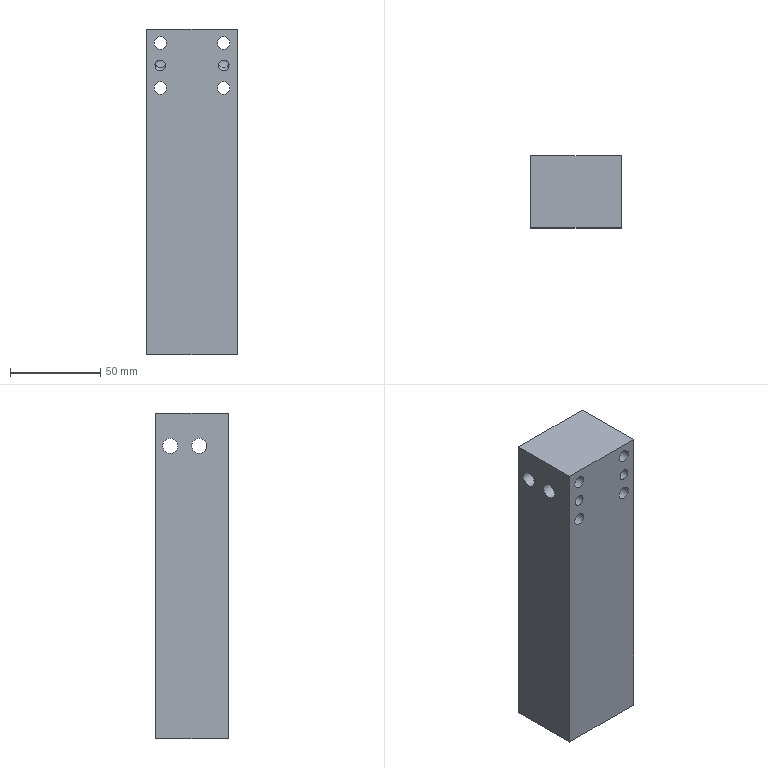Part | NX | features BREP 1 | 1 solid | 24 faces | box 50 x 40 x 180 mm | volume 345283 mm3 | cylinder 12 | plane 6 | cone 6 | commonest cylinder face diameters 6 x4 7 x4 6.8 x2 8.5 x2
STEP:
#1=CARTESIAN_POINT('',(25.,12.,67.75));
#2=VERTEX_POINT('',#1);
#3=CARTESIAN_POINT('',(25.,12.,72.));
#4=DIRECTION('',(1.,0.,0.));
#5=DIRECTION('',(0.,0.,-1.));
#6=AXIS2_PLACEMENT_3D('',#3,#4,#5);
#7=CIRCLE('',#6,4.25);
#8=EDGE_CURVE('',#2,#2,#7,.T.);
#9=ORIENTED_EDGE('',*,*,#8,.F.);
#10=EDGE_LOOP('',(#9));
#11=FACE_BOUND('',#10,.T.);
#12=CARTESIAN_POINT('',(25.,-4.,67.75));
#13=VERTEX_POINT('',#12);
#14=CARTESIAN_POINT('',(25.,-4.,72.));
#15=DIRECTION('',(1.,0.,0.));
#16=DIRECTION('',(0.,0.,-1.));
#17=AXIS2_PLACEMENT_3D('',#14,#15,#16);
#18=CIRCLE('',#17,4.25);
#19=EDGE_CURVE('',#13,#13,#18,.T.);
#20=ORIENTED_EDGE('',*,*,#19,.F.);
#21=EDGE_LOOP('',(#20));
#22=FACE_BOUND('',#21,.T.);
#23=CARTESIAN_POINT('',(25.,-20.,90.));
#24=VERTEX_POINT('',#23);
#25=CARTESIAN_POINT('',(25.,-20.,-90.));
#26=VERTEX_POINT('',#25);
#27=CARTESIAN_POINT('',(25.,-20.,90.));
#28=DIRECTION('',(0.,0.,-1.));
#29=VECTOR('',#28,1000.);
#30=LINE('',#27,#29);
#31=EDGE_CURVE('',#24,#26,#30,.T.);
#32=ORIENTED_EDGE('',*,*,#31,.T.);
#33=CARTESIAN_POINT('',(25.,20.,-90.));
#34=VERTEX_POINT('',#33);
#35=CARTESIAN_POINT('',(25.,20.,-90.));
#36=DIRECTION('',(0.,-1.,0.));
#37=VECTOR('',#36,1000.);
#38=LINE('',#35,#37);
#39=EDGE_CURVE('',#34,#26,#38,.T.);
#40=ORIENTED_EDGE('',*,*,#39,.F.);
#41=CARTESIAN_POINT('',(25.,20.,90.));
#42=VERTEX_POINT('',#41);
#43=CARTESIAN_POINT('',(25.,20.,90.));
#44=DIRECTION('',(0.,0.,-1.));
#45=VECTOR('',#44,1000.);
#46=LINE('',#43,#45);
#47=EDGE_CURVE('',#42,#34,#46,.T.);
#48=ORIENTED_EDGE('',*,*,#47,.F.);
#49=CARTESIAN_POINT('',(25.,20.,90.));
#50=DIRECTION('',(0.,-1.,0.));
#51=VECTOR('',#50,1000.);
#52=LINE('',#49,#51);
#53=EDGE_CURVE('',#42,#24,#52,.T.);
#54=ORIENTED_EDGE('',*,*,#53,.T.);
#55=EDGE_LOOP('',(#32,#40,#48,#54));
#56=FACE_BOUND('',#55,.T.);
#57=CARTESIAN_POINT('',(25.,20.,90.));
#58=DIRECTION('',(-1.,0.,0.));
#59=DIRECTION('',(0.,0.,-1.));
#60=AXIS2_PLACEMENT_3D('',#57,#58,#59);
#61=PLANE('',#60);
#62=ADVANCED_FACE('',(#11,#22,#56),#61,.F.);
#63=CARTESIAN_POINT('',(9.5,10.,-90.));
#64=VERTEX_POINT('',#63);
#65=CARTESIAN_POINT('',(12.5,10.,-90.));
#66=DIRECTION('',(0.,0.,-1.));
#67=DIRECTION('',(-1.,0.,0.));
#68=AXIS2_PLACEMENT_3D('',#65,#66,#67);
#69=CIRCLE('',#68,3.);
#70=EDGE_CURVE('',#64,#64,#69,.T.);
#71=ORIENTED_EDGE('',*,*,#70,.F.);
#72=EDGE_LOOP('',(#71));
#73=FACE_BOUND('',#72,.T.);
#74=CARTESIAN_POINT('',(-15.5,-10.,-90.));
#75=VERTEX_POINT('',#74);
#76=CARTESIAN_POINT('',(-12.5,-10.,-90.));
#77=DIRECTION('',(0.,0.,-1.));
#78=DIRECTION('',(-1.,0.,0.));
#79=AXIS2_PLACEMENT_3D('',#76,#77,#78);
#80=CIRCLE('',#79,3.);
#81=EDGE_CURVE('',#75,#75,#80,.T.);
#82=ORIENTED_EDGE('',*,*,#81,.F.);
#83=EDGE_LOOP('',(#82));
#84=FACE_BOUND('',#83,.T.);
#85=CARTESIAN_POINT('',(-15.9,10.,-90.));
#86=VERTEX_POINT('',#85);
#87=CARTESIAN_POINT('',(-12.5,10.,-90.));
#88=DIRECTION('',(0.,0.,-1.));
#89=DIRECTION('',(-1.,0.,0.));
#90=AXIS2_PLACEMENT_3D('',#87,#88,#89);
#91=CIRCLE('',#90,3.4);
#92=EDGE_CURVE('',#86,#86,#91,.T.);
#93=ORIENTED_EDGE('',*,*,#92,.F.);
#94=EDGE_LOOP('',(#93));
#95=FACE_BOUND('',#94,.T.);
#96=CARTESIAN_POINT('',(9.1,-10.,-90.));
#97=VERTEX_POINT('',#96);
#98=CARTESIAN_POINT('',(12.5,-10.,-90.));
#99=DIRECTION('',(0.,0.,-1.));
#100=DIRECTION('',(-1.,0.,0.));
#101=AXIS2_PLACEMENT_3D('',#98,#99,#100);
#102=CIRCLE('',#101,3.4);
#103=EDGE_CURVE('',#97,#97,#102,.T.);
#104=ORIENTED_EDGE('',*,*,#103,.F.);
#105=EDGE_LOOP('',(#104));
#106=FACE_BOUND('',#105,.T.);
#107=CARTESIAN_POINT('',(-25.,-20.,-90.));
#108=VERTEX_POINT('',#107);
#109=CARTESIAN_POINT('',(-25.,-20.,-90.));
#110=DIRECTION('',(-1.,0.,0.));
#111=VECTOR('',#110,1000.);
#112=LINE('',#109,#111);
#113=EDGE_CURVE('',#26,#108,#112,.T.);
#114=ORIENTED_EDGE('',*,*,#113,.T.);
#115=CARTESIAN_POINT('',(-25.,20.,-90.));
#116=VERTEX_POINT('',#115);
#117=CARTESIAN_POINT('',(-25.,20.,-90.));
#118=DIRECTION('',(0.,-1.,0.));
#119=VECTOR('',#118,1000.);
#120=LINE('',#117,#119);
#121=EDGE_CURVE('',#116,#108,#120,.T.);
#122=ORIENTED_EDGE('',*,*,#121,.F.);
#123=CARTESIAN_POINT('',(-25.,20.,-90.));
#124=DIRECTION('',(-1.,0.,0.));
#125=VECTOR('',#124,1000.);
#126=LINE('',#123,#125);
#127=EDGE_CURVE('',#34,#116,#126,.T.);
#128=ORIENTED_EDGE('',*,*,#127,.F.);
#129=ORIENTED_EDGE('',*,*,#39,.T.);
#130=EDGE_LOOP('',(#114,#122,#128,#129));
#131=FACE_BOUND('',#130,.T.);
#132=CARTESIAN_POINT('',(-25.,20.,-90.));
#133=DIRECTION('',(0.,0.,1.));
#134=DIRECTION('',(-1.,0.,0.));
#135=AXIS2_PLACEMENT_3D('',#132,#133,#134);
#136=PLANE('',#135);
#137=ADVANCED_FACE('',(#73,#84,#95,#106,#131),#136,.F.);
#138=CARTESIAN_POINT('',(-25.,12.,67.75));
#139=VERTEX_POINT('',#138);
#140=CARTESIAN_POINT('',(-25.,12.,72.));
#141=DIRECTION('',(1.,0.,0.));
#142=DIRECTION('',(0.,0.,-1.));
#143=AXIS2_PLACEMENT_3D('',#140,#141,#142);
#144=CIRCLE('',#143,4.25);
#145=EDGE_CURVE('',#139,#139,#144,.T.);
#146=ORIENTED_EDGE('',*,*,#145,.T.);
#147=EDGE_LOOP('',(#146));
#148=FACE_BOUND('',#147,.T.);
#149=CARTESIAN_POINT('',(-25.,-4.,67.75));
#150=VERTEX_POINT('',#149);
#151=CARTESIAN_POINT('',(-25.,-4.,72.));
#152=DIRECTION('',(1.,0.,0.));
#153=DIRECTION('',(0.,0.,-1.));
#154=AXIS2_PLACEMENT_3D('',#151,#152,#153);
#155=CIRCLE('',#154,4.25);
#156=EDGE_CURVE('',#150,#150,#155,.T.);
#157=ORIENTED_EDGE('',*,*,#156,.T.);
#158=EDGE_LOOP('',(#157));
#159=FACE_BOUND('',#158,.T.);
#160=CARTESIAN_POINT('',(-25.,-20.,90.));
#161=VERTEX_POINT('',#160);
#162=CARTESIAN_POINT('',(-25.,-20.,90.));
#163=DIRECTION('',(0.,0.,1.));
#164=VECTOR('',#163,1000.);
#165=LINE('',#162,#164);
#166=EDGE_CURVE('',#108,#161,#165,.T.);
#167=ORIENTED_EDGE('',*,*,#166,.T.);
#168=CARTESIAN_POINT('',(-25.,20.,90.));
#169=VERTEX_POINT('',#168);
#170=CARTESIAN_POINT('',(-25.,20.,90.));
#171=DIRECTION('',(0.,-1.,0.));
#172=VECTOR('',#171,1000.);
#173=LINE('',#170,#172);
#174=EDGE_CURVE('',#169,#161,#173,.T.);
#175=ORIENTED_EDGE('',*,*,#174,.F.);
#176=CARTESIAN_POINT('',(-25.,20.,90.));
#177=DIRECTION('',(0.,0.,1.));
#178=VECTOR('',#177,1000.);
#179=LINE('',#176,#178);
#180=EDGE_CURVE('',#116,#169,#179,.T.);
#181=ORIENTED_EDGE('',*,*,#180,.F.);
#182=ORIENTED_EDGE('',*,*,#121,.T.);
#183=EDGE_LOOP('',(#167,#175,#181,#182));
#184=FACE_BOUND('',#183,.T.);
#185=CARTESIAN_POINT('',(-25.,20.,90.));
#186=DIRECTION('',(1.,0.,0.));
#187=DIRECTION('',(0.,0.,1.));
#188=AXIS2_PLACEMENT_3D('',#185,#186,#187);
#189=PLANE('',#188);
#190=ADVANCED_FACE('',(#148,#159,#184),#189,.F.);
#191=CARTESIAN_POINT('',(-25.,-20.,90.));
#192=DIRECTION('',(1.,0.,0.));
#193=VECTOR('',#192,1000.);
#194=LINE('',#191,#193);
#195=EDGE_CURVE('',#161,#24,#194,.T.);
#196=ORIENTED_EDGE('',*,*,#195,.T.);
#197=ORIENTED_EDGE('',*,*,#53,.F.);
#198=CARTESIAN_POINT('',(-25.,20.,90.));
#199=DIRECTION('',(1.,0.,0.));
#200=VECTOR('',#199,1000.);
#201=LINE('',#198,#200);
#202=EDGE_CURVE('',#169,#42,#201,.T.);
#203=ORIENTED_EDGE('',*,*,#202,.F.);
#204=ORIENTED_EDGE('',*,*,#174,.T.);
#205=EDGE_LOOP('',(#196,#197,#203,#204));
#206=FACE_BOUND('',#205,.T.);
#207=CARTESIAN_POINT('',(-25.,20.,90.));
#208=DIRECTION('',(0.,0.,-1.));
#209=DIRECTION('',(1.,0.,0.));
#210=AXIS2_PLACEMENT_3D('',#207,#208,#209);
#211=PLANE('',#210);
#212=ADVANCED_FACE('',(#206),#211,.F.);
#213=CARTESIAN_POINT('',(17.5,20.,86.));
#214=VERTEX_POINT('',#213);
#215=CARTESIAN_POINT('',(17.5,20.,82.5));
#216=DIRECTION('',(0.,1.,0.));
#217=DIRECTION('',(0.,0.,1.));
#218=AXIS2_PLACEMENT_3D('',#215,#216,#217);
#219=CIRCLE('',#218,3.5);
#220=EDGE_CURVE('',#214,#214,#219,.T.);
#221=ORIENTED_EDGE('',*,*,#220,.F.);
#222=EDGE_LOOP('',(#221));
#223=FACE_BOUND('',#222,.T.);
#224=CARTESIAN_POINT('',(17.5,20.,61.));
#225=VERTEX_POINT('',#224);
#226=CARTESIAN_POINT('',(17.5,20.,57.5));
#227=DIRECTION('',(0.,1.,0.));
#228=DIRECTION('',(0.,0.,1.));
#229=AXIS2_PLACEMENT_3D('',#226,#227,#228);
#230=CIRCLE('',#229,3.5);
#231=EDGE_CURVE('',#225,#225,#230,.T.);
#232=ORIENTED_EDGE('',*,*,#231,.F.);
#233=EDGE_LOOP('',(#232));
#234=FACE_BOUND('',#233,.T.);
#235=CARTESIAN_POINT('',(-17.5,20.,61.));
#236=VERTEX_POINT('',#235);
#237=CARTESIAN_POINT('',(-17.5,20.,57.5));
#238=DIRECTION('',(0.,1.,0.));
#239=DIRECTION('',(0.,0.,1.));
#240=AXIS2_PLACEMENT_3D('',#237,#238,#239);
#241=CIRCLE('',#240,3.5);
#242=EDGE_CURVE('',#236,#236,#241,.T.);
#243=ORIENTED_EDGE('',*,*,#242,.F.);
#244=EDGE_LOOP('',(#243));
#245=FACE_BOUND('',#244,.T.);
#246=CARTESIAN_POINT('',(-17.5,20.,86.));
#247=VERTEX_POINT('',#246);
#248=CARTESIAN_POINT('',(-17.5,20.,82.5));
#249=DIRECTION('',(0.,1.,0.));
#250=DIRECTION('',(0.,0.,1.));
#251=AXIS2_PLACEMENT_3D('',#248,#249,#250);
#252=CIRCLE('',#251,3.5);
#253=EDGE_CURVE('',#247,#247,#252,.T.);
#254=ORIENTED_EDGE('',*,*,#253,.F.);
#255=EDGE_LOOP('',(#254));
#256=FACE_BOUND('',#255,.T.);
#257=ORIENTED_EDGE('',*,*,#47,.T.);
#258=ORIENTED_EDGE('',*,*,#127,.T.);
#259=ORIENTED_EDGE('',*,*,#180,.T.);
#260=ORIENTED_EDGE('',*,*,#202,.T.);
#261=EDGE_LOOP('',(#257,#258,#259,#260));
#262=FACE_BOUND('',#261,.T.);
#263=CARTESIAN_POINT('',(0.,20.,0.));
#264=DIRECTION('',(0.,-1.,0.));
#265=DIRECTION('',(0.,0.,1.));
#266=AXIS2_PLACEMENT_3D('',#263,#264,#265);
#267=PLANE('',#266);
#268=ADVANCED_FACE('',(#223,#234,#245,#256,#262),#267,.F.);
#269=CARTESIAN_POINT('',(-17.5,-20.,67.));
#270=VERTEX_POINT('',#269);
#271=CARTESIAN_POINT('',(-17.5,-20.,70.));
#272=DIRECTION('',(0.,-1.,0.));
#273=DIRECTION('',(0.,0.,-1.));
#274=AXIS2_PLACEMENT_3D('',#271,#272,#273);
#275=CIRCLE('',#274,3.);
#276=EDGE_CURVE('',#270,#270,#275,.T.);
#277=ORIENTED_EDGE('',*,*,#276,.F.);
#278=EDGE_LOOP('',(#277));
#279=FACE_BOUND('',#278,.T.);
#280=CARTESIAN_POINT('',(17.5,-20.,67.));
#281=VERTEX_POINT('',#280);
#282=CARTESIAN_POINT('',(17.5,-20.,70.));
#283=DIRECTION('',(0.,-1.,0.));
#284=DIRECTION('',(0.,0.,-1.));
#285=AXIS2_PLACEMENT_3D('',#282,#283,#284);
#286=CIRCLE('',#285,3.);
#287=EDGE_CURVE('',#281,#281,#286,.T.);
#288=ORIENTED_EDGE('',*,*,#287,.F.);
#289=EDGE_LOOP('',(#288));
#290=FACE_BOUND('',#289,.T.);
#291=CARTESIAN_POINT('',(17.5,-20.,86.));
#292=VERTEX_POINT('',#291);
#293=CARTESIAN_POINT('',(17.5,-20.,82.5));
#294=DIRECTION('',(0.,1.,0.));
#295=DIRECTION('',(0.,0.,1.));
#296=AXIS2_PLACEMENT_3D('',#293,#294,#295);
#297=CIRCLE('',#296,3.5);
#298=EDGE_CURVE('',#292,#292,#297,.T.);
#299=ORIENTED_EDGE('',*,*,#298,.T.);
#300=EDGE_LOOP('',(#299));
#301=FACE_BOUND('',#300,.T.);
#302=CARTESIAN_POINT('',(17.5,-20.,61.));
#303=VERTEX_POINT('',#302);
#304=CARTESIAN_POINT('',(17.5,-20.,57.5));
#305=DIRECTION('',(0.,1.,0.));
#306=DIRECTION('',(0.,0.,1.));
#307=AXIS2_PLACEMENT_3D('',#304,#305,#306);
#308=CIRCLE('',#307,3.5);
#309=EDGE_CURVE('',#303,#303,#308,.T.);
#310=ORIENTED_EDGE('',*,*,#309,.T.);
#311=EDGE_LOOP('',(#310));
#312=FACE_BOUND('',#311,.T.);
#313=CARTESIAN_POINT('',(-17.5,-20.,61.));
#314=VERTEX_POINT('',#313);
#315=CARTESIAN_POINT('',(-17.5,-20.,57.5));
#316=DIRECTION('',(0.,1.,0.));
#317=DIRECTION('',(0.,0.,1.));
#318=AXIS2_PLACEMENT_3D('',#315,#316,#317);
#319=CIRCLE('',#318,3.5);
#320=EDGE_CURVE('',#314,#314,#319,.T.);
#321=ORIENTED_EDGE('',*,*,#320,.T.);
#322=EDGE_LOOP('',(#321));
#323=FACE_BOUND('',#322,.T.);
#324=CARTESIAN_POINT('',(-17.5,-20.,86.));
#325=VERTEX_POINT('',#324);
#326=CARTESIAN_POINT('',(-17.5,-20.,82.5));
#327=DIRECTION('',(0.,1.,0.));
#328=DIRECTION('',(0.,0.,1.));
#329=AXIS2_PLACEMENT_3D('',#326,#327,#328);
#330=CIRCLE('',#329,3.5);
#331=EDGE_CURVE('',#325,#325,#330,.T.);
#332=ORIENTED_EDGE('',*,*,#331,.T.);
#333=EDGE_LOOP('',(#332));
#334=FACE_BOUND('',#333,.T.);
#335=ORIENTED_EDGE('',*,*,#31,.F.);
#336=ORIENTED_EDGE('',*,*,#195,.F.);
#337=ORIENTED_EDGE('',*,*,#166,.F.);
#338=ORIENTED_EDGE('',*,*,#113,.F.);
#339=EDGE_LOOP('',(#335,#336,#337,#338));
#340=FACE_BOUND('',#339,.T.);
#341=CARTESIAN_POINT('',(0.,-20.,0.));
#342=DIRECTION('',(0.,-1.,0.));
#343=DIRECTION('',(0.,0.,1.));
#344=AXIS2_PLACEMENT_3D('',#341,#342,#343);
#345=PLANE('',#344);
#346=ADVANCED_FACE('',(#279,#290,#301,#312,#323,#334,#340),#345,.T.);
#347=ORIENTED_EDGE('',*,*,#331,.F.);
#348=EDGE_LOOP('',(#347));
#349=FACE_BOUND('',#348,.T.);
#350=ORIENTED_EDGE('',*,*,#253,.T.);
#351=EDGE_LOOP('',(#350));
#352=FACE_BOUND('',#351,.T.);
#353=CARTESIAN_POINT('',(-17.5,20.,82.5));
#354=DIRECTION('',(0.,1.,0.));
#355=DIRECTION('',(0.,0.,-1.));
#356=AXIS2_PLACEMENT_3D('',#353,#354,#355);
#357=CYLINDRICAL_SURFACE('',#356,3.5);
#358=ADVANCED_FACE('',(#349,#352),#357,.F.);
#359=ORIENTED_EDGE('',*,*,#320,.F.);
#360=EDGE_LOOP('',(#359));
#361=FACE_BOUND('',#360,.T.);
#362=ORIENTED_EDGE('',*,*,#242,.T.);
#363=EDGE_LOOP('',(#362));
#364=FACE_BOUND('',#363,.T.);
#365=CARTESIAN_POINT('',(-17.5,20.,57.5));
#366=DIRECTION('',(0.,1.,0.));
#367=DIRECTION('',(0.,0.,-1.));
#368=AXIS2_PLACEMENT_3D('',#365,#366,#367);
#369=CYLINDRICAL_SURFACE('',#368,3.5);
#370=ADVANCED_FACE('',(#361,#364),#369,.F.);
#371=ORIENTED_EDGE('',*,*,#309,.F.);
#372=EDGE_LOOP('',(#371));
#373=FACE_BOUND('',#372,.T.);
#374=ORIENTED_EDGE('',*,*,#231,.T.);
#375=EDGE_LOOP('',(#374));
#376=FACE_BOUND('',#375,.T.);
#377=CARTESIAN_POINT('',(17.5,20.,57.5));
#378=DIRECTION('',(0.,1.,0.));
#379=DIRECTION('',(0.,0.,-1.));
#380=AXIS2_PLACEMENT_3D('',#377,#378,#379);
#381=CYLINDRICAL_SURFACE('',#380,3.5);
#382=ADVANCED_FACE('',(#373,#376),#381,.F.);
#383=ORIENTED_EDGE('',*,*,#298,.F.);
#384=EDGE_LOOP('',(#383));
#385=FACE_BOUND('',#384,.T.);
#386=ORIENTED_EDGE('',*,*,#220,.T.);
#387=EDGE_LOOP('',(#386));
#388=FACE_BOUND('',#387,.T.);
#389=CARTESIAN_POINT('',(17.5,20.,82.5));
#390=DIRECTION('',(0.,1.,0.));
#391=DIRECTION('',(0.,0.,-1.));
#392=AXIS2_PLACEMENT_3D('',#389,#390,#391);
#393=CYLINDRICAL_SURFACE('',#392,3.5);
#394=ADVANCED_FACE('',(#385,#388),#393,.F.);
#395=CARTESIAN_POINT('',(12.5,-10.,-68.207));
#396=VERTEX_POINT('',#395);
#397=VERTEX_LOOP('',#396);
#398=FACE_BOUND('',#397,.T.);
#399=CARTESIAN_POINT('',(9.1,-10.,-70.25));
#400=VERTEX_POINT('',#399);
#401=CARTESIAN_POINT('',(12.5,-10.,-70.25));
#402=DIRECTION('',(0.,0.,-1.));
#403=DIRECTION('',(-1.,0.,0.));
#404=AXIS2_PLACEMENT_3D('',#401,#402,#403);
#405=CIRCLE('',#404,3.4);
#406=EDGE_CURVE('',#400,#400,#405,.T.);
#407=ORIENTED_EDGE('',*,*,#406,.T.);
#408=EDGE_LOOP('',(#407));
#409=FACE_BOUND('',#408,.T.);
#410=CARTESIAN_POINT('',(12.5,-10.,-70.25));
#411=DIRECTION('',(0.,0.,-1.));
#412=DIRECTION('',(1.,0.,0.));
#413=AXIS2_PLACEMENT_3D('',#410,#411,#412);
#414=CONICAL_SURFACE('',#413,3.4,1.03);
#415=ADVANCED_FACE('',(#398,#409),#414,.F.);
#416=ORIENTED_EDGE('',*,*,#406,.F.);
#417=EDGE_LOOP('',(#416));
#418=FACE_BOUND('',#417,.T.);
#419=ORIENTED_EDGE('',*,*,#103,.T.);
#420=EDGE_LOOP('',(#419));
#421=FACE_BOUND('',#420,.T.);
#422=CARTESIAN_POINT('',(12.5,-10.,-90.));
#423=DIRECTION('',(0.,0.,-1.));
#424=DIRECTION('',(1.,0.,0.));
#425=AXIS2_PLACEMENT_3D('',#422,#423,#424);
#426=CYLINDRICAL_SURFACE('',#425,3.4);
#427=ADVANCED_FACE('',(#418,#421),#426,.F.);
#428=CARTESIAN_POINT('',(-12.5,10.,-68.207));
#429=VERTEX_POINT('',#428);
#430=VERTEX_LOOP('',#429);
#431=FACE_BOUND('',#430,.T.);
#432=CARTESIAN_POINT('',(-15.9,10.,-70.25));
#433=VERTEX_POINT('',#432);
#434=CARTESIAN_POINT('',(-12.5,10.,-70.25));
#435=DIRECTION('',(0.,0.,-1.));
#436=DIRECTION('',(-1.,0.,0.));
#437=AXIS2_PLACEMENT_3D('',#434,#435,#436);
#438=CIRCLE('',#437,3.4);
#439=EDGE_CURVE('',#433,#433,#438,.T.);
#440=ORIENTED_EDGE('',*,*,#439,.T.);
#441=EDGE_LOOP('',(#440));
#442=FACE_BOUND('',#441,.T.);
#443=CARTESIAN_POINT('',(-12.5,10.,-70.25));
#444=DIRECTION('',(0.,0.,-1.));
#445=DIRECTION('',(1.,0.,0.));
#446=AXIS2_PLACEMENT_3D('',#443,#444,#445);
#447=CONICAL_SURFACE('',#446,3.4,1.03);
#448=ADVANCED_FACE('',(#431,#442),#447,.F.);
#449=ORIENTED_EDGE('',*,*,#439,.F.);
#450=EDGE_LOOP('',(#449));
#451=FACE_BOUND('',#450,.T.);
#452=ORIENTED_EDGE('',*,*,#92,.T.);
#453=EDGE_LOOP('',(#452));
#454=FACE_BOUND('',#453,.T.);
#455=CARTESIAN_POINT('',(-12.5,10.,-90.));
#456=DIRECTION('',(0.,0.,-1.));
#457=DIRECTION('',(1.,0.,0.));
#458=AXIS2_PLACEMENT_3D('',#455,#456,#457);
#459=CYLINDRICAL_SURFACE('',#458,3.4);
#460=ADVANCED_FACE('',(#451,#454),#459,.F.);
#461=CARTESIAN_POINT('',(14.553,-8.,70.564));
#462=VERTEX_POINT('',#461);
#463=CARTESIAN_POINT('',(20.447,-8.,70.564));
#464=VERTEX_POINT('',#463);
#465=CARTESIAN_POINT('',(17.5,-8.,70.));
#466=DIRECTION('',(0.,-1.,0.));
#467=DIRECTION('',(0.,0.,-1.));
#468=AXIS2_PLACEMENT_3D('',#465,#466,#467);
#469=CIRCLE('',#468,3.);
#470=EDGE_CURVE('',#462,#464,#469,.T.);
#471=ORIENTED_EDGE('',*,*,#470,.T.);
#472=CARTESIAN_POINT('',(20.447,-8.,70.564));
#473=CARTESIAN_POINT('',(20.214,-7.8,70.007));
#474=CARTESIAN_POINT('',(19.317,-7.293,69.243));
#475=CARTESIAN_POINT('',(17.511,-6.669,68.686));
#476=CARTESIAN_POINT('',(15.688,-7.288,69.237));
#477=CARTESIAN_POINT('',(14.786,-7.8,70.006));
#478=CARTESIAN_POINT('',(14.553,-8.,70.564));
#479=B_SPLINE_CURVE_WITH_KNOTS('',3,(#472,#473,#474,#475,#476,#477,#478),.UNSPECIFIED.,.F.,.F.,(4,1,1,1,4),(0.,0.001872,0.003744,0.005615,0.007487),.UNSPECIFIED.);
#480=EDGE_CURVE('',#464,#462,#479,.T.);
#481=ORIENTED_EDGE('',*,*,#480,.T.);
#482=EDGE_LOOP('',(#471,#481));
#483=FACE_BOUND('',#482,.T.);
#484=CARTESIAN_POINT('',(17.5,-8.,70.));
#485=DIRECTION('',(0.,-1.,0.));
#486=DIRECTION('',(0.,0.,1.));
#487=AXIS2_PLACEMENT_3D('',#484,#485,#486);
#488=CONICAL_SURFACE('',#487,3.,1.03);
#489=ADVANCED_FACE('',(#483),#488,.F.);
#490=ORIENTED_EDGE('',*,*,#470,.F.);
#491=CARTESIAN_POINT('',(14.553,-8.,70.564));
#492=CARTESIAN_POINT('',(14.678,-8.234,71.215));
#493=CARTESIAN_POINT('',(15.418,-8.296,72.503));
#494=CARTESIAN_POINT('',(17.501,-8.048,73.249));
#495=CARTESIAN_POINT('',(19.582,-8.296,72.503));
#496=CARTESIAN_POINT('',(20.322,-8.234,71.215));
#497=CARTESIAN_POINT('',(20.447,-8.,70.564));
#498=B_SPLINE_CURVE_WITH_KNOTS('',3,(#491,#492,#493,#494,#495,#496,#497),.UNSPECIFIED.,.F.,.F.,(4,1,1,1,4),(0.,0.002078,0.004155,0.006233,0.008311),.UNSPECIFIED.);
#499=EDGE_CURVE('',#462,#464,#498,.T.);
#500=ORIENTED_EDGE('',*,*,#499,.T.);
#501=EDGE_LOOP('',(#490,#500));
#502=FACE_BOUND('',#501,.T.);
#503=ORIENTED_EDGE('',*,*,#287,.T.);
#504=EDGE_LOOP('',(#503));
#505=FACE_BOUND('',#504,.T.);
#506=CARTESIAN_POINT('',(17.5,-20.,70.));
#507=DIRECTION('',(0.,-1.,0.));
#508=DIRECTION('',(0.,0.,1.));
#509=AXIS2_PLACEMENT_3D('',#506,#507,#508);
#510=CYLINDRICAL_SURFACE('',#509,3.);
#511=ADVANCED_FACE('',(#502,#505),#510,.F.);
#512=CARTESIAN_POINT('',(-20.447,-8.,70.564));
#513=VERTEX_POINT('',#512);
#514=CARTESIAN_POINT('',(-14.553,-8.,70.564));
#515=VERTEX_POINT('',#514);
#516=CARTESIAN_POINT('',(-17.5,-8.,70.));
#517=DIRECTION('',(0.,-1.,0.));
#518=DIRECTION('',(0.,0.,-1.));
#519=AXIS2_PLACEMENT_3D('',#516,#517,#518);
#520=CIRCLE('',#519,3.);
#521=EDGE_CURVE('',#513,#515,#520,.T.);
#522=ORIENTED_EDGE('',*,*,#521,.T.);
#523=CARTESIAN_POINT('',(-14.553,-8.,70.564));
#524=CARTESIAN_POINT('',(-14.786,-7.8,70.007));
#525=CARTESIAN_POINT('',(-15.683,-7.293,69.243));
#526=CARTESIAN_POINT('',(-17.489,-6.669,68.686));
#527=CARTESIAN_POINT('',(-19.312,-7.288,69.237));
#528=CARTESIAN_POINT('',(-20.214,-7.8,70.006));
#529=CARTESIAN_POINT('',(-20.447,-8.,70.564));
#530=B_SPLINE_CURVE_WITH_KNOTS('',3,(#523,#524,#525,#526,#527,#528,#529),.UNSPECIFIED.,.F.,.F.,(4,1,1,1,4),(0.,0.001872,0.003744,0.005615,0.007487),.UNSPECIFIED.);
#531=EDGE_CURVE('',#515,#513,#530,.T.);
#532=ORIENTED_EDGE('',*,*,#531,.T.);
#533=EDGE_LOOP('',(#522,#532));
#534=FACE_BOUND('',#533,.T.);
#535=CARTESIAN_POINT('',(-17.5,-8.,70.));
#536=DIRECTION('',(0.,-1.,0.));
#537=DIRECTION('',(0.,0.,1.));
#538=AXIS2_PLACEMENT_3D('',#535,#536,#537);
#539=CONICAL_SURFACE('',#538,3.,1.03);
#540=ADVANCED_FACE('',(#534),#539,.F.);
#541=ORIENTED_EDGE('',*,*,#521,.F.);
#542=CARTESIAN_POINT('',(-20.447,-8.,70.564));
#543=CARTESIAN_POINT('',(-20.322,-8.234,71.215));
#544=CARTESIAN_POINT('',(-19.582,-8.296,72.503));
#545=CARTESIAN_POINT('',(-17.499,-8.048,73.249));
#546=CARTESIAN_POINT('',(-15.418,-8.296,72.503));
#547=CARTESIAN_POINT('',(-14.678,-8.234,71.215));
#548=CARTESIAN_POINT('',(-14.553,-8.,70.564));
#549=B_SPLINE_CURVE_WITH_KNOTS('',3,(#542,#543,#544,#545,#546,#547,#548),.UNSPECIFIED.,.F.,.F.,(4,1,1,1,4),(0.,0.002078,0.004155,0.006233,0.008311),.UNSPECIFIED.);
#550=EDGE_CURVE('',#513,#515,#549,.T.);
#551=ORIENTED_EDGE('',*,*,#550,.T.);
#552=EDGE_LOOP('',(#541,#551));
#553=FACE_BOUND('',#552,.T.);
#554=ORIENTED_EDGE('',*,*,#276,.T.);
#555=EDGE_LOOP('',(#554));
#556=FACE_BOUND('',#555,.T.);
#557=CARTESIAN_POINT('',(-17.5,-20.,70.));
#558=DIRECTION('',(0.,-1.,0.));
#559=DIRECTION('',(0.,0.,1.));
#560=AXIS2_PLACEMENT_3D('',#557,#558,#559);
#561=CYLINDRICAL_SURFACE('',#560,3.);
#562=ADVANCED_FACE('',(#553,#556),#561,.F.);
#563=CARTESIAN_POINT('',(-12.5,-10.,-76.197));
#564=VERTEX_POINT('',#563);
#565=VERTEX_LOOP('',#564);
#566=FACE_BOUND('',#565,.T.);
#567=CARTESIAN_POINT('',(-15.5,-10.,-78.));
#568=VERTEX_POINT('',#567);
#569=CARTESIAN_POINT('',(-12.5,-10.,-78.));
#570=DIRECTION('',(0.,0.,-1.));
#571=DIRECTION('',(-1.,0.,0.));
#572=AXIS2_PLACEMENT_3D('',#569,#570,#571);
#573=CIRCLE('',#572,3.);
#574=EDGE_CURVE('',#568,#568,#573,.T.);
#575=ORIENTED_EDGE('',*,*,#574,.T.);
#576=EDGE_LOOP('',(#575));
#577=FACE_BOUND('',#576,.T.);
#578=CARTESIAN_POINT('',(-12.5,-10.,-78.));
#579=DIRECTION('',(0.,0.,-1.));
#580=DIRECTION('',(1.,0.,0.));
#581=AXIS2_PLACEMENT_3D('',#578,#579,#580);
#582=CONICAL_SURFACE('',#581,3.,1.03);
#583=ADVANCED_FACE('',(#566,#577),#582,.F.);
#584=ORIENTED_EDGE('',*,*,#574,.F.);
#585=EDGE_LOOP('',(#584));
#586=FACE_BOUND('',#585,.T.);
#587=ORIENTED_EDGE('',*,*,#81,.T.);
#588=EDGE_LOOP('',(#587));
#589=FACE_BOUND('',#588,.T.);
#590=CARTESIAN_POINT('',(-12.5,-10.,-90.));
#591=DIRECTION('',(0.,0.,-1.));
#592=DIRECTION('',(1.,0.,0.));
#593=AXIS2_PLACEMENT_3D('',#590,#591,#592);
#594=CYLINDRICAL_SURFACE('',#593,3.);
#595=ADVANCED_FACE('',(#586,#589),#594,.F.);
#596=CARTESIAN_POINT('',(12.5,10.,-76.197));
#597=VERTEX_POINT('',#596);
#598=VERTEX_LOOP('',#597);
#599=FACE_BOUND('',#598,.T.);
#600=CARTESIAN_POINT('',(9.5,10.,-78.));
#601=VERTEX_POINT('',#600);
#602=CARTESIAN_POINT('',(12.5,10.,-78.));
#603=DIRECTION('',(0.,0.,-1.));
#604=DIRECTION('',(-1.,0.,0.));
#605=AXIS2_PLACEMENT_3D('',#602,#603,#604);
#606=CIRCLE('',#605,3.);
#607=EDGE_CURVE('',#601,#601,#606,.T.);
#608=ORIENTED_EDGE('',*,*,#607,.T.);
#609=EDGE_LOOP('',(#608));
#610=FACE_BOUND('',#609,.T.);
#611=CARTESIAN_POINT('',(12.5,10.,-78.));
#612=DIRECTION('',(0.,0.,-1.));
#613=DIRECTION('',(1.,0.,0.));
#614=AXIS2_PLACEMENT_3D('',#611,#612,#613);
#615=CONICAL_SURFACE('',#614,3.,1.03);
#616=ADVANCED_FACE('',(#599,#610),#615,.F.);
#617=ORIENTED_EDGE('',*,*,#607,.F.);
#618=EDGE_LOOP('',(#617));
#619=FACE_BOUND('',#618,.T.);
#620=ORIENTED_EDGE('',*,*,#70,.T.);
#621=EDGE_LOOP('',(#620));
#622=FACE_BOUND('',#621,.T.);
#623=CARTESIAN_POINT('',(12.5,10.,-90.));
#624=DIRECTION('',(0.,0.,-1.));
#625=DIRECTION('',(1.,0.,0.));
#626=AXIS2_PLACEMENT_3D('',#623,#624,#625);
#627=CYLINDRICAL_SURFACE('',#626,3.);
#628=ADVANCED_FACE('',(#619,#622),#627,.F.);
#629=ORIENTED_EDGE('',*,*,#156,.F.);
#630=EDGE_LOOP('',(#629));
#631=FACE_BOUND('',#630,.T.);
#632=ORIENTED_EDGE('',*,*,#19,.T.);
#633=EDGE_LOOP('',(#632));
#634=FACE_BOUND('',#633,.T.);
#635=ORIENTED_EDGE('',*,*,#480,.F.);
#636=ORIENTED_EDGE('',*,*,#499,.F.);
#637=EDGE_LOOP('',(#635,#636));
#638=FACE_BOUND('',#637,.T.);
#639=ORIENTED_EDGE('',*,*,#531,.F.);
#640=ORIENTED_EDGE('',*,*,#550,.F.);
#641=EDGE_LOOP('',(#639,#640));
#642=FACE_BOUND('',#641,.T.);
#643=CARTESIAN_POINT('',(25.,-4.,72.));
#644=DIRECTION('',(1.,0.,0.));
#645=DIRECTION('',(0.,0.,1.));
#646=AXIS2_PLACEMENT_3D('',#643,#644,#645);
#647=CYLINDRICAL_SURFACE('',#646,4.25);
#648=ADVANCED_FACE('',(#631,#634,#638,#642),#647,.F.);
#649=ORIENTED_EDGE('',*,*,#145,.F.);
#650=EDGE_LOOP('',(#649));
#651=FACE_BOUND('',#650,.T.);
#652=ORIENTED_EDGE('',*,*,#8,.T.);
#653=EDGE_LOOP('',(#652));
#654=FACE_BOUND('',#653,.T.);
#655=CARTESIAN_POINT('',(25.,12.,72.));
#656=DIRECTION('',(1.,0.,0.));
#657=DIRECTION('',(0.,0.,1.));
#658=AXIS2_PLACEMENT_3D('',#655,#656,#657);
#659=CYLINDRICAL_SURFACE('',#658,4.25);
#660=ADVANCED_FACE('',(#651,#654),#659,.F.);
#661=CLOSED_SHELL('',(#62,#137,#190,#212,#268,#346,#358,#370,#382,#394,#415,#427,#448,#460,#489,#511,#540,#562,#583,#595,#616,#628,#648,#660));
#662=MANIFOLD_SOLID_BREP('',#661);
#663=(LENGTH_UNIT()NAMED_UNIT(*)SI_UNIT(.MILLI.,.METRE.));
#664=UNCERTAINTY_MEASURE_WITH_UNIT(LENGTH_MEASURE(0.0508),#663,'','');
#665=(NAMED_UNIT(*)PLANE_ANGLE_UNIT()SI_UNIT($,.RADIAN.));
#666=(NAMED_UNIT(*)SI_UNIT($,.STERADIAN.)SOLID_ANGLE_UNIT());
#667=(GEOMETRIC_REPRESENTATION_CONTEXT(3)GLOBAL_UNCERTAINTY_ASSIGNED_CONTEXT((#664))GLOBAL_UNIT_ASSIGNED_CONTEXT((#663,#665,#666))REPRESENTATION_CONTEXT('',''));
#668=ADVANCED_BREP_SHAPE_REPRESENTATION('',(#662),#667);